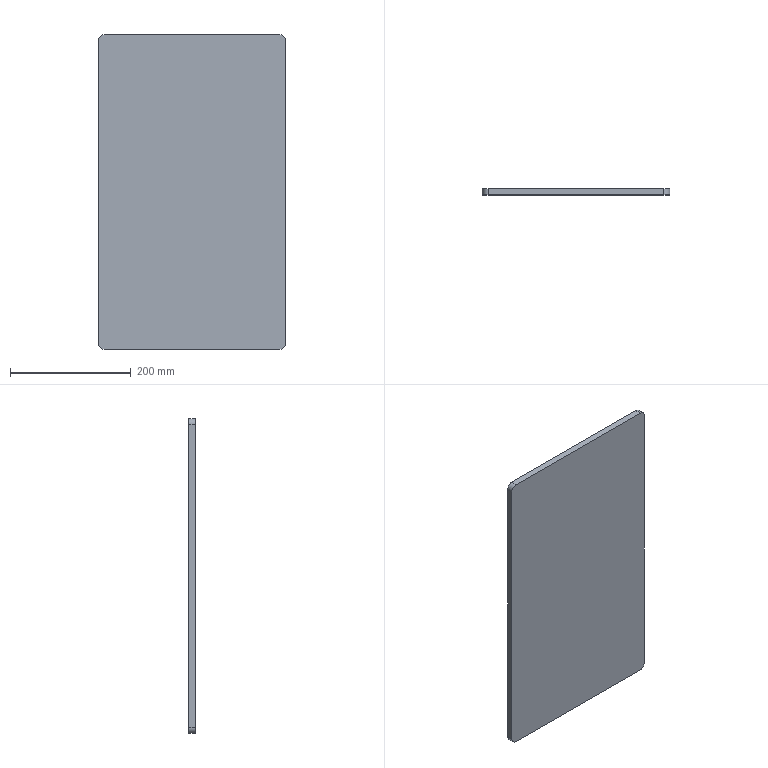Part | SolidWorks | features BaseBody 1 | 1 solid | 10 faces | box 310 x 10 x 520 mm | volume 1611142 mm3 | plane 6 | cylinder 4 | commonest cylinder face diameters 20 x4
STEP:
#1=CARTESIAN_POINT('',(-155.,10.,250.));
#2=VERTEX_POINT('',#1);
#3=CARTESIAN_POINT('',(-145.,10.,260.));
#4=VERTEX_POINT('',#3);
#5=CARTESIAN_POINT('',(-145.,10.,250.));
#6=DIRECTION('',(0.,1.,0.));
#7=DIRECTION('',(0.,0.,1.));
#8=AXIS2_PLACEMENT_3D('',#5,#6,#7);
#9=CIRCLE('',#8,10.);
#10=EDGE_CURVE('',#2,#4,#9,.T.);
#11=ORIENTED_EDGE('',*,*,#10,.F.);
#12=CARTESIAN_POINT('',(-155.,0.,250.));
#13=VERTEX_POINT('',#12);
#14=CARTESIAN_POINT('',(-155.,10.,250.));
#15=DIRECTION('',(0.,1.,0.));
#16=VECTOR('',#15,1000.);
#17=LINE('',#14,#16);
#18=EDGE_CURVE('',#13,#2,#17,.T.);
#19=ORIENTED_EDGE('',*,*,#18,.F.);
#20=CARTESIAN_POINT('',(-145.,0.,260.));
#21=VERTEX_POINT('',#20);
#22=CARTESIAN_POINT('',(-145.,0.,250.));
#23=DIRECTION('',(0.,-1.,0.));
#24=DIRECTION('',(0.,0.,1.));
#25=AXIS2_PLACEMENT_3D('',#22,#23,#24);
#26=CIRCLE('',#25,10.);
#27=EDGE_CURVE('',#21,#13,#26,.T.);
#28=ORIENTED_EDGE('',*,*,#27,.F.);
#29=CARTESIAN_POINT('',(-145.,10.,260.));
#30=DIRECTION('',(0.,-1.,0.));
#31=VECTOR('',#30,1000.);
#32=LINE('',#29,#31);
#33=EDGE_CURVE('',#4,#21,#32,.T.);
#34=ORIENTED_EDGE('',*,*,#33,.F.);
#35=EDGE_LOOP('',(#11,#19,#28,#34));
#36=FACE_OUTER_BOUND('',#35,.T.);
#37=CARTESIAN_POINT('',(-145.,10.,250.));
#38=DIRECTION('',(0.,-1.,0.));
#39=DIRECTION('',(0.,0.,-1.));
#40=AXIS2_PLACEMENT_3D('',#37,#38,#39);
#41=CYLINDRICAL_SURFACE('',#40,10.);
#42=ADVANCED_FACE('',(#36),#41,.T.);
#43=CARTESIAN_POINT('',(145.,10.,260.));
#44=VERTEX_POINT('',#43);
#45=CARTESIAN_POINT('',(155.,10.,250.));
#46=VERTEX_POINT('',#45);
#47=CARTESIAN_POINT('',(145.,10.,250.));
#48=DIRECTION('',(0.,1.,0.));
#49=DIRECTION('',(0.,0.,1.));
#50=AXIS2_PLACEMENT_3D('',#47,#48,#49);
#51=CIRCLE('',#50,10.);
#52=EDGE_CURVE('',#44,#46,#51,.T.);
#53=ORIENTED_EDGE('',*,*,#52,.F.);
#54=CARTESIAN_POINT('',(145.,0.,260.));
#55=VERTEX_POINT('',#54);
#56=CARTESIAN_POINT('',(145.,10.,260.));
#57=DIRECTION('',(0.,1.,0.));
#58=VECTOR('',#57,1000.);
#59=LINE('',#56,#58);
#60=EDGE_CURVE('',#55,#44,#59,.T.);
#61=ORIENTED_EDGE('',*,*,#60,.F.);
#62=CARTESIAN_POINT('',(155.,0.,250.));
#63=VERTEX_POINT('',#62);
#64=CARTESIAN_POINT('',(145.,0.,250.));
#65=DIRECTION('',(0.,-1.,0.));
#66=DIRECTION('',(0.,0.,1.));
#67=AXIS2_PLACEMENT_3D('',#64,#65,#66);
#68=CIRCLE('',#67,10.);
#69=EDGE_CURVE('',#63,#55,#68,.T.);
#70=ORIENTED_EDGE('',*,*,#69,.F.);
#71=CARTESIAN_POINT('',(155.,10.,250.));
#72=DIRECTION('',(0.,-1.,0.));
#73=VECTOR('',#72,1000.);
#74=LINE('',#71,#73);
#75=EDGE_CURVE('',#46,#63,#74,.T.);
#76=ORIENTED_EDGE('',*,*,#75,.F.);
#77=EDGE_LOOP('',(#53,#61,#70,#76));
#78=FACE_OUTER_BOUND('',#77,.T.);
#79=CARTESIAN_POINT('',(145.,10.,250.));
#80=DIRECTION('',(0.,-1.,0.));
#81=DIRECTION('',(0.,0.,-1.));
#82=AXIS2_PLACEMENT_3D('',#79,#80,#81);
#83=CYLINDRICAL_SURFACE('',#82,10.);
#84=ADVANCED_FACE('',(#78),#83,.T.);
#85=CARTESIAN_POINT('',(-145.,10.,-260.));
#86=VERTEX_POINT('',#85);
#87=CARTESIAN_POINT('',(-155.,10.,-250.));
#88=VERTEX_POINT('',#87);
#89=CARTESIAN_POINT('',(-145.,10.,-250.));
#90=DIRECTION('',(0.,1.,0.));
#91=DIRECTION('',(0.,0.,1.));
#92=AXIS2_PLACEMENT_3D('',#89,#90,#91);
#93=CIRCLE('',#92,10.);
#94=EDGE_CURVE('',#86,#88,#93,.T.);
#95=ORIENTED_EDGE('',*,*,#94,.F.);
#96=CARTESIAN_POINT('',(-145.,0.,-260.));
#97=VERTEX_POINT('',#96);
#98=CARTESIAN_POINT('',(-145.,10.,-260.));
#99=DIRECTION('',(0.,1.,0.));
#100=VECTOR('',#99,1000.);
#101=LINE('',#98,#100);
#102=EDGE_CURVE('',#97,#86,#101,.T.);
#103=ORIENTED_EDGE('',*,*,#102,.F.);
#104=CARTESIAN_POINT('',(-155.,0.,-250.));
#105=VERTEX_POINT('',#104);
#106=CARTESIAN_POINT('',(-145.,0.,-250.));
#107=DIRECTION('',(0.,-1.,0.));
#108=DIRECTION('',(0.,0.,1.));
#109=AXIS2_PLACEMENT_3D('',#106,#107,#108);
#110=CIRCLE('',#109,10.);
#111=EDGE_CURVE('',#105,#97,#110,.T.);
#112=ORIENTED_EDGE('',*,*,#111,.F.);
#113=CARTESIAN_POINT('',(-155.,10.,-250.));
#114=DIRECTION('',(0.,-1.,0.));
#115=VECTOR('',#114,1000.);
#116=LINE('',#113,#115);
#117=EDGE_CURVE('',#88,#105,#116,.T.);
#118=ORIENTED_EDGE('',*,*,#117,.F.);
#119=EDGE_LOOP('',(#95,#103,#112,#118));
#120=FACE_OUTER_BOUND('',#119,.T.);
#121=CARTESIAN_POINT('',(-145.,10.,-250.));
#122=DIRECTION('',(0.,-1.,0.));
#123=DIRECTION('',(0.,0.,-1.));
#124=AXIS2_PLACEMENT_3D('',#121,#122,#123);
#125=CYLINDRICAL_SURFACE('',#124,10.);
#126=ADVANCED_FACE('',(#120),#125,.T.);
#127=CARTESIAN_POINT('',(155.,10.,-250.));
#128=VERTEX_POINT('',#127);
#129=CARTESIAN_POINT('',(145.,10.,-260.));
#130=VERTEX_POINT('',#129);
#131=CARTESIAN_POINT('',(145.,10.,-250.));
#132=DIRECTION('',(0.,1.,0.));
#133=DIRECTION('',(0.,0.,1.));
#134=AXIS2_PLACEMENT_3D('',#131,#132,#133);
#135=CIRCLE('',#134,10.);
#136=EDGE_CURVE('',#128,#130,#135,.T.);
#137=ORIENTED_EDGE('',*,*,#136,.F.);
#138=CARTESIAN_POINT('',(155.,0.,-250.));
#139=VERTEX_POINT('',#138);
#140=CARTESIAN_POINT('',(155.,10.,-250.));
#141=DIRECTION('',(0.,1.,0.));
#142=VECTOR('',#141,1000.);
#143=LINE('',#140,#142);
#144=EDGE_CURVE('',#139,#128,#143,.T.);
#145=ORIENTED_EDGE('',*,*,#144,.F.);
#146=CARTESIAN_POINT('',(145.,0.,-260.));
#147=VERTEX_POINT('',#146);
#148=CARTESIAN_POINT('',(145.,0.,-250.));
#149=DIRECTION('',(0.,-1.,0.));
#150=DIRECTION('',(0.,0.,1.));
#151=AXIS2_PLACEMENT_3D('',#148,#149,#150);
#152=CIRCLE('',#151,10.);
#153=EDGE_CURVE('',#147,#139,#152,.T.);
#154=ORIENTED_EDGE('',*,*,#153,.F.);
#155=CARTESIAN_POINT('',(145.,10.,-260.));
#156=DIRECTION('',(0.,-1.,0.));
#157=VECTOR('',#156,1000.);
#158=LINE('',#155,#157);
#159=EDGE_CURVE('',#130,#147,#158,.T.);
#160=ORIENTED_EDGE('',*,*,#159,.F.);
#161=EDGE_LOOP('',(#137,#145,#154,#160));
#162=FACE_OUTER_BOUND('',#161,.T.);
#163=CARTESIAN_POINT('',(145.,10.,-250.));
#164=DIRECTION('',(0.,-1.,0.));
#165=DIRECTION('',(0.,0.,-1.));
#166=AXIS2_PLACEMENT_3D('',#163,#164,#165);
#167=CYLINDRICAL_SURFACE('',#166,10.);
#168=ADVANCED_FACE('',(#162),#167,.T.);
#169=CARTESIAN_POINT('',(-155.,0.,-260.));
#170=DIRECTION('',(-1.,0.,0.));
#171=VECTOR('',#170,1000.);
#172=LINE('',#169,#171);
#173=EDGE_CURVE('',#147,#97,#172,.T.);
#174=ORIENTED_EDGE('',*,*,#173,.F.);
#175=ORIENTED_EDGE('',*,*,#153,.T.);
#176=CARTESIAN_POINT('',(155.,0.,-260.));
#177=DIRECTION('',(0.,0.,-1.));
#178=VECTOR('',#177,1000.);
#179=LINE('',#176,#178);
#180=EDGE_CURVE('',#63,#139,#179,.T.);
#181=ORIENTED_EDGE('',*,*,#180,.F.);
#182=ORIENTED_EDGE('',*,*,#69,.T.);
#183=CARTESIAN_POINT('',(-155.,0.,260.));
#184=DIRECTION('',(1.,0.,0.));
#185=VECTOR('',#184,1000.);
#186=LINE('',#183,#185);
#187=EDGE_CURVE('',#21,#55,#186,.T.);
#188=ORIENTED_EDGE('',*,*,#187,.F.);
#189=ORIENTED_EDGE('',*,*,#27,.T.);
#190=CARTESIAN_POINT('',(-155.,0.,-260.));
#191=DIRECTION('',(0.,0.,1.));
#192=VECTOR('',#191,1000.);
#193=LINE('',#190,#192);
#194=EDGE_CURVE('',#105,#13,#193,.T.);
#195=ORIENTED_EDGE('',*,*,#194,.F.);
#196=ORIENTED_EDGE('',*,*,#111,.T.);
#197=EDGE_LOOP('',(#174,#175,#181,#182,#188,#189,#195,#196));
#198=FACE_OUTER_BOUND('',#197,.T.);
#199=CARTESIAN_POINT('',(0.,0.,0.));
#200=DIRECTION('',(0.,1.,0.));
#201=DIRECTION('',(1.,0.,0.));
#202=AXIS2_PLACEMENT_3D('',#199,#200,#201);
#203=PLANE('',#202);
#204=ADVANCED_FACE('',(#198),#203,.F.);
#205=CARTESIAN_POINT('',(155.,10.,-260.));
#206=DIRECTION('',(0.,0.,-1.));
#207=VECTOR('',#206,1000.);
#208=LINE('',#205,#207);
#209=EDGE_CURVE('',#46,#128,#208,.T.);
#210=ORIENTED_EDGE('',*,*,#209,.T.);
#211=ORIENTED_EDGE('',*,*,#136,.T.);
#212=CARTESIAN_POINT('',(-155.,10.,-260.));
#213=DIRECTION('',(-1.,0.,0.));
#214=VECTOR('',#213,1000.);
#215=LINE('',#212,#214);
#216=EDGE_CURVE('',#130,#86,#215,.T.);
#217=ORIENTED_EDGE('',*,*,#216,.T.);
#218=ORIENTED_EDGE('',*,*,#94,.T.);
#219=CARTESIAN_POINT('',(-155.,10.,-260.));
#220=DIRECTION('',(0.,0.,1.));
#221=VECTOR('',#220,1000.);
#222=LINE('',#219,#221);
#223=EDGE_CURVE('',#88,#2,#222,.T.);
#224=ORIENTED_EDGE('',*,*,#223,.T.);
#225=ORIENTED_EDGE('',*,*,#10,.T.);
#226=CARTESIAN_POINT('',(-155.,10.,260.));
#227=DIRECTION('',(1.,0.,0.));
#228=VECTOR('',#227,1000.);
#229=LINE('',#226,#228);
#230=EDGE_CURVE('',#4,#44,#229,.T.);
#231=ORIENTED_EDGE('',*,*,#230,.T.);
#232=ORIENTED_EDGE('',*,*,#52,.T.);
#233=EDGE_LOOP('',(#210,#211,#217,#218,#224,#225,#231,#232));
#234=FACE_OUTER_BOUND('',#233,.T.);
#235=CARTESIAN_POINT('',(0.,10.,0.));
#236=DIRECTION('',(0.,1.,0.));
#237=DIRECTION('',(1.,0.,0.));
#238=AXIS2_PLACEMENT_3D('',#235,#236,#237);
#239=PLANE('',#238);
#240=ADVANCED_FACE('',(#234),#239,.T.);
#241=ORIENTED_EDGE('',*,*,#187,.T.);
#242=ORIENTED_EDGE('',*,*,#60,.T.);
#243=ORIENTED_EDGE('',*,*,#230,.F.);
#244=ORIENTED_EDGE('',*,*,#33,.T.);
#245=EDGE_LOOP('',(#241,#242,#243,#244));
#246=FACE_OUTER_BOUND('',#245,.T.);
#247=CARTESIAN_POINT('',(-155.,10.,260.));
#248=DIRECTION('',(0.,0.,-1.));
#249=DIRECTION('',(0.,-1.,0.));
#250=AXIS2_PLACEMENT_3D('',#247,#248,#249);
#251=PLANE('',#250);
#252=ADVANCED_FACE('',(#246),#251,.F.);
#253=ORIENTED_EDGE('',*,*,#223,.F.);
#254=ORIENTED_EDGE('',*,*,#117,.T.);
#255=ORIENTED_EDGE('',*,*,#194,.T.);
#256=ORIENTED_EDGE('',*,*,#18,.T.);
#257=EDGE_LOOP('',(#253,#254,#255,#256));
#258=FACE_OUTER_BOUND('',#257,.T.);
#259=CARTESIAN_POINT('',(-155.,10.,-260.));
#260=DIRECTION('',(1.,0.,0.));
#261=DIRECTION('',(0.,0.,-1.));
#262=AXIS2_PLACEMENT_3D('',#259,#260,#261);
#263=PLANE('',#262);
#264=ADVANCED_FACE('',(#258),#263,.F.);
#265=ORIENTED_EDGE('',*,*,#216,.F.);
#266=ORIENTED_EDGE('',*,*,#159,.T.);
#267=ORIENTED_EDGE('',*,*,#173,.T.);
#268=ORIENTED_EDGE('',*,*,#102,.T.);
#269=EDGE_LOOP('',(#265,#266,#267,#268));
#270=FACE_OUTER_BOUND('',#269,.T.);
#271=CARTESIAN_POINT('',(-155.,10.,-260.));
#272=DIRECTION('',(0.,0.,1.));
#273=DIRECTION('',(1.,0.,0.));
#274=AXIS2_PLACEMENT_3D('',#271,#272,#273);
#275=PLANE('',#274);
#276=ADVANCED_FACE('',(#270),#275,.F.);
#277=ORIENTED_EDGE('',*,*,#180,.T.);
#278=ORIENTED_EDGE('',*,*,#144,.T.);
#279=ORIENTED_EDGE('',*,*,#209,.F.);
#280=ORIENTED_EDGE('',*,*,#75,.T.);
#281=EDGE_LOOP('',(#277,#278,#279,#280));
#282=FACE_OUTER_BOUND('',#281,.T.);
#283=CARTESIAN_POINT('',(155.,10.,-260.));
#284=DIRECTION('',(-1.,0.,0.));
#285=DIRECTION('',(0.,1.,0.));
#286=AXIS2_PLACEMENT_3D('',#283,#284,#285);
#287=PLANE('',#286);
#288=ADVANCED_FACE('',(#282),#287,.F.);
#289=CLOSED_SHELL('',(#42,#84,#126,#168,#204,#240,#252,#264,#276,#288));
#290=MANIFOLD_SOLID_BREP('',#289);
#291=CARTESIAN_POINT('',(0.,0.,0.));
#292=DIRECTION('',(0.,0.,1.));
#293=DIRECTION('',(1.,0.,0.));
#294=AXIS2_PLACEMENT_3D('',#291,#292,#293);
#295=(LENGTH_UNIT()NAMED_UNIT(*)SI_UNIT(.MILLI.,.METRE.));
#296=UNCERTAINTY_MEASURE_WITH_UNIT(LENGTH_MEASURE(0.00001),#295,'','');
#297=(NAMED_UNIT(*)PLANE_ANGLE_UNIT()SI_UNIT($,.RADIAN.));
#298=(NAMED_UNIT(*)SI_UNIT($,.STERADIAN.)SOLID_ANGLE_UNIT());
#299=(GEOMETRIC_REPRESENTATION_CONTEXT(3)GLOBAL_UNCERTAINTY_ASSIGNED_CONTEXT((#296))GLOBAL_UNIT_ASSIGNED_CONTEXT((#295,#297,#298))REPRESENTATION_CONTEXT('',''));
#300=ADVANCED_BREP_SHAPE_REPRESENTATION('',(#290,#294),#299);